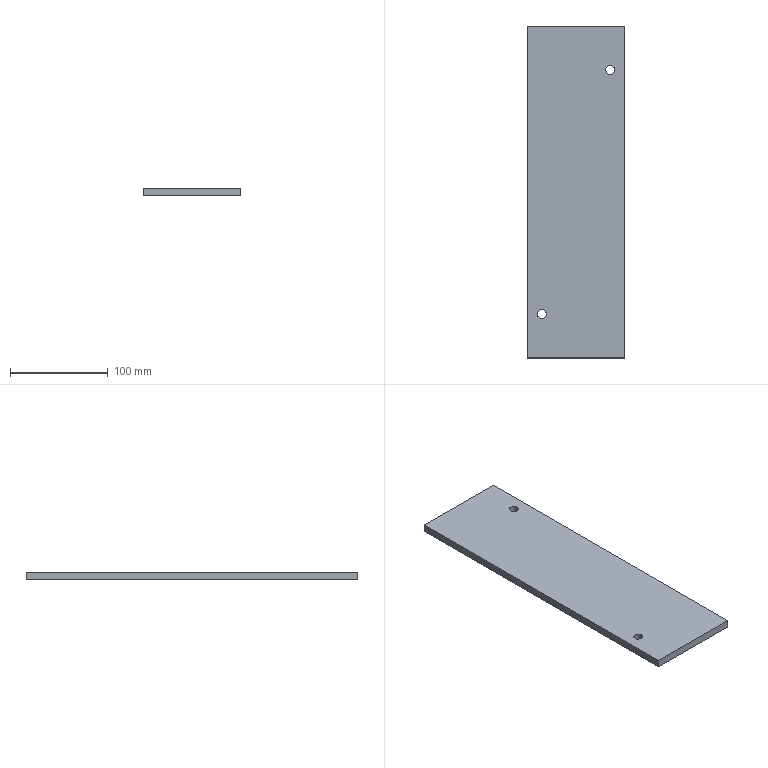Part | SolidWorks | features Extrusion 1, ICE 1 | 1 solid | 10 faces | box 100 x 340 x 8 mm | volume 270982 mm3 | plane 6 | cylinder 4 | commonest cylinder face diameters 9 x4
STEP:
#1=CARTESIAN_POINT('',(-39.5,-125.,-4.));
#2=VERTEX_POINT('',#1);
#3=CARTESIAN_POINT('',(-30.5,-125.,-4.));
#4=VERTEX_POINT('',#3);
#5=CARTESIAN_POINT('',(-35.,-125.,-4.));
#6=DIRECTION('',(0.,0.,1.));
#7=DIRECTION('',(1.,0.,0.));
#8=AXIS2_PLACEMENT_3D('',#5,#6,#7);
#9=CIRCLE('',#8,4.5);
#10=EDGE_CURVE('',#2,#4,#9,.T.);
#11=ORIENTED_EDGE('',*,*,#10,.F.);
#12=CARTESIAN_POINT('',(-39.5,-125.,4.));
#13=VERTEX_POINT('',#12);
#14=CARTESIAN_POINT('',(-39.5,-125.,-14.));
#15=DIRECTION('',(0.,0.,1.));
#16=VECTOR('',#15,1000.);
#17=LINE('',#14,#16);
#18=EDGE_CURVE('',#2,#13,#17,.T.);
#19=ORIENTED_EDGE('',*,*,#18,.T.);
#20=CARTESIAN_POINT('',(-30.5,-125.,4.));
#21=VERTEX_POINT('',#20);
#22=CARTESIAN_POINT('',(-35.,-125.,4.));
#23=DIRECTION('',(0.,0.,1.));
#24=DIRECTION('',(1.,0.,0.));
#25=AXIS2_PLACEMENT_3D('',#22,#23,#24);
#26=CIRCLE('',#25,4.5);
#27=EDGE_CURVE('',#13,#21,#26,.T.);
#28=ORIENTED_EDGE('',*,*,#27,.T.);
#29=CARTESIAN_POINT('',(-30.5,-125.,-14.));
#30=DIRECTION('',(0.,0.,1.));
#31=VECTOR('',#30,1000.);
#32=LINE('',#29,#31);
#33=EDGE_CURVE('',#4,#21,#32,.T.);
#34=ORIENTED_EDGE('',*,*,#33,.F.);
#35=EDGE_LOOP('',(#11,#19,#28,#34));
#36=FACE_OUTER_BOUND('',#35,.T.);
#37=CARTESIAN_POINT('',(-35.,-125.,-14.));
#38=DIRECTION('',(0.,0.,1.));
#39=DIRECTION('',(1.,0.,0.));
#40=AXIS2_PLACEMENT_3D('',#37,#38,#39);
#41=CYLINDRICAL_SURFACE('',#40,4.5);
#42=ADVANCED_FACE('',(#36),#41,.F.);
#43=CARTESIAN_POINT('',(30.5,125.,-4.));
#44=VERTEX_POINT('',#43);
#45=CARTESIAN_POINT('',(39.5,125.,-4.));
#46=VERTEX_POINT('',#45);
#47=CARTESIAN_POINT('',(35.,125.,-4.));
#48=DIRECTION('',(0.,0.,1.));
#49=DIRECTION('',(1.,0.,0.));
#50=AXIS2_PLACEMENT_3D('',#47,#48,#49);
#51=CIRCLE('',#50,4.5);
#52=EDGE_CURVE('',#44,#46,#51,.T.);
#53=ORIENTED_EDGE('',*,*,#52,.F.);
#54=CARTESIAN_POINT('',(30.5,125.,4.));
#55=VERTEX_POINT('',#54);
#56=CARTESIAN_POINT('',(30.5,125.,-14.));
#57=DIRECTION('',(0.,0.,1.));
#58=VECTOR('',#57,1000.);
#59=LINE('',#56,#58);
#60=EDGE_CURVE('',#44,#55,#59,.T.);
#61=ORIENTED_EDGE('',*,*,#60,.T.);
#62=CARTESIAN_POINT('',(39.5,125.,4.));
#63=VERTEX_POINT('',#62);
#64=CARTESIAN_POINT('',(35.,125.,4.));
#65=DIRECTION('',(0.,0.,1.));
#66=DIRECTION('',(1.,0.,0.));
#67=AXIS2_PLACEMENT_3D('',#64,#65,#66);
#68=CIRCLE('',#67,4.5);
#69=EDGE_CURVE('',#55,#63,#68,.T.);
#70=ORIENTED_EDGE('',*,*,#69,.T.);
#71=CARTESIAN_POINT('',(39.5,125.,-14.));
#72=DIRECTION('',(0.,0.,1.));
#73=VECTOR('',#72,1000.);
#74=LINE('',#71,#73);
#75=EDGE_CURVE('',#46,#63,#74,.T.);
#76=ORIENTED_EDGE('',*,*,#75,.F.);
#77=EDGE_LOOP('',(#53,#61,#70,#76));
#78=FACE_OUTER_BOUND('',#77,.T.);
#79=CARTESIAN_POINT('',(35.,125.,-14.));
#80=DIRECTION('',(0.,0.,1.));
#81=DIRECTION('',(1.,0.,0.));
#82=AXIS2_PLACEMENT_3D('',#79,#80,#81);
#83=CYLINDRICAL_SURFACE('',#82,4.5);
#84=ADVANCED_FACE('',(#78),#83,.F.);
#85=CARTESIAN_POINT('',(-50.,170.,4.));
#86=VERTEX_POINT('',#85);
#87=CARTESIAN_POINT('',(-50.,-170.,4.));
#88=VERTEX_POINT('',#87);
#89=CARTESIAN_POINT('',(-50.,170.,4.));
#90=DIRECTION('',(0.,-1.,0.));
#91=VECTOR('',#90,1000.);
#92=LINE('',#89,#91);
#93=EDGE_CURVE('',#86,#88,#92,.T.);
#94=ORIENTED_EDGE('',*,*,#93,.F.);
#95=CARTESIAN_POINT('',(-50.,170.,-4.));
#96=VERTEX_POINT('',#95);
#97=CARTESIAN_POINT('',(-50.,170.,-4.));
#98=DIRECTION('',(0.,0.,1.));
#99=VECTOR('',#98,1000.);
#100=LINE('',#97,#99);
#101=EDGE_CURVE('',#96,#86,#100,.T.);
#102=ORIENTED_EDGE('',*,*,#101,.F.);
#103=CARTESIAN_POINT('',(-50.,-170.,-4.));
#104=VERTEX_POINT('',#103);
#105=CARTESIAN_POINT('',(-50.,170.,-4.));
#106=DIRECTION('',(0.,-1.,0.));
#107=VECTOR('',#106,1000.);
#108=LINE('',#105,#107);
#109=EDGE_CURVE('',#96,#104,#108,.T.);
#110=ORIENTED_EDGE('',*,*,#109,.T.);
#111=CARTESIAN_POINT('',(-50.,-170.,-4.));
#112=DIRECTION('',(0.,0.,1.));
#113=VECTOR('',#112,1000.);
#114=LINE('',#111,#113);
#115=EDGE_CURVE('',#104,#88,#114,.T.);
#116=ORIENTED_EDGE('',*,*,#115,.T.);
#117=EDGE_LOOP('',(#94,#102,#110,#116));
#118=FACE_OUTER_BOUND('',#117,.T.);
#119=CARTESIAN_POINT('',(-50.,170.,-4.));
#120=DIRECTION('',(-1.,0.,0.));
#121=DIRECTION('',(0.,0.,1.));
#122=AXIS2_PLACEMENT_3D('',#119,#120,#121);
#123=PLANE('',#122);
#124=ADVANCED_FACE('',(#118),#123,.T.);
#125=CARTESIAN_POINT('',(50.,170.,4.));
#126=VERTEX_POINT('',#125);
#127=CARTESIAN_POINT('',(50.,170.,4.));
#128=DIRECTION('',(-1.,0.,0.));
#129=VECTOR('',#128,1000.);
#130=LINE('',#127,#129);
#131=EDGE_CURVE('',#126,#86,#130,.T.);
#132=ORIENTED_EDGE('',*,*,#131,.F.);
#133=CARTESIAN_POINT('',(50.,170.,-4.));
#134=VERTEX_POINT('',#133);
#135=CARTESIAN_POINT('',(50.,170.,-4.));
#136=DIRECTION('',(0.,0.,1.));
#137=VECTOR('',#136,1000.);
#138=LINE('',#135,#137);
#139=EDGE_CURVE('',#134,#126,#138,.T.);
#140=ORIENTED_EDGE('',*,*,#139,.F.);
#141=CARTESIAN_POINT('',(50.,170.,-4.));
#142=DIRECTION('',(-1.,0.,0.));
#143=VECTOR('',#142,1000.);
#144=LINE('',#141,#143);
#145=EDGE_CURVE('',#134,#96,#144,.T.);
#146=ORIENTED_EDGE('',*,*,#145,.T.);
#147=ORIENTED_EDGE('',*,*,#101,.T.);
#148=EDGE_LOOP('',(#132,#140,#146,#147));
#149=FACE_OUTER_BOUND('',#148,.T.);
#150=CARTESIAN_POINT('',(50.,170.,-4.));
#151=DIRECTION('',(0.,1.,0.));
#152=DIRECTION('',(0.,0.,1.));
#153=AXIS2_PLACEMENT_3D('',#150,#151,#152);
#154=PLANE('',#153);
#155=ADVANCED_FACE('',(#149),#154,.T.);
#156=CARTESIAN_POINT('',(50.,-170.,4.));
#157=VERTEX_POINT('',#156);
#158=CARTESIAN_POINT('',(50.,-170.,4.));
#159=DIRECTION('',(0.,1.,0.));
#160=VECTOR('',#159,1000.);
#161=LINE('',#158,#160);
#162=EDGE_CURVE('',#157,#126,#161,.T.);
#163=ORIENTED_EDGE('',*,*,#162,.F.);
#164=CARTESIAN_POINT('',(50.,-170.,-4.));
#165=VERTEX_POINT('',#164);
#166=CARTESIAN_POINT('',(50.,-170.,-4.));
#167=DIRECTION('',(0.,0.,1.));
#168=VECTOR('',#167,1000.);
#169=LINE('',#166,#168);
#170=EDGE_CURVE('',#165,#157,#169,.T.);
#171=ORIENTED_EDGE('',*,*,#170,.F.);
#172=CARTESIAN_POINT('',(50.,-170.,-4.));
#173=DIRECTION('',(0.,1.,0.));
#174=VECTOR('',#173,1000.);
#175=LINE('',#172,#174);
#176=EDGE_CURVE('',#165,#134,#175,.T.);
#177=ORIENTED_EDGE('',*,*,#176,.T.);
#178=ORIENTED_EDGE('',*,*,#139,.T.);
#179=EDGE_LOOP('',(#163,#171,#177,#178));
#180=FACE_OUTER_BOUND('',#179,.T.);
#181=CARTESIAN_POINT('',(50.,-170.,-4.));
#182=DIRECTION('',(1.,0.,0.));
#183=DIRECTION('',(0.,0.,-1.));
#184=AXIS2_PLACEMENT_3D('',#181,#182,#183);
#185=PLANE('',#184);
#186=ADVANCED_FACE('',(#180),#185,.T.);
#187=CARTESIAN_POINT('',(-50.,-170.,4.));
#188=DIRECTION('',(1.,0.,0.));
#189=VECTOR('',#188,1000.);
#190=LINE('',#187,#189);
#191=EDGE_CURVE('',#88,#157,#190,.T.);
#192=ORIENTED_EDGE('',*,*,#191,.F.);
#193=ORIENTED_EDGE('',*,*,#115,.F.);
#194=CARTESIAN_POINT('',(-50.,-170.,-4.));
#195=DIRECTION('',(1.,0.,0.));
#196=VECTOR('',#195,1000.);
#197=LINE('',#194,#196);
#198=EDGE_CURVE('',#104,#165,#197,.T.);
#199=ORIENTED_EDGE('',*,*,#198,.T.);
#200=ORIENTED_EDGE('',*,*,#170,.T.);
#201=EDGE_LOOP('',(#192,#193,#199,#200));
#202=FACE_OUTER_BOUND('',#201,.T.);
#203=CARTESIAN_POINT('',(-50.,-170.,-4.));
#204=DIRECTION('',(0.,-1.,0.));
#205=DIRECTION('',(0.,0.,-1.));
#206=AXIS2_PLACEMENT_3D('',#203,#204,#205);
#207=PLANE('',#206);
#208=ADVANCED_FACE('',(#202),#207,.T.);
#209=CARTESIAN_POINT('',(-35.,-125.,-4.));
#210=DIRECTION('',(0.,0.,1.));
#211=DIRECTION('',(1.,0.,0.));
#212=AXIS2_PLACEMENT_3D('',#209,#210,#211);
#213=CIRCLE('',#212,4.5);
#214=EDGE_CURVE('',#4,#2,#213,.T.);
#215=ORIENTED_EDGE('',*,*,#214,.T.);
#216=ORIENTED_EDGE('',*,*,#10,.T.);
#217=EDGE_LOOP('',(#215,#216));
#218=FACE_BOUND('',#217,.T.);
#219=CARTESIAN_POINT('',(35.,125.,-4.));
#220=DIRECTION('',(0.,0.,1.));
#221=DIRECTION('',(1.,0.,0.));
#222=AXIS2_PLACEMENT_3D('',#219,#220,#221);
#223=CIRCLE('',#222,4.5);
#224=EDGE_CURVE('',#46,#44,#223,.T.);
#225=ORIENTED_EDGE('',*,*,#224,.T.);
#226=ORIENTED_EDGE('',*,*,#52,.T.);
#227=EDGE_LOOP('',(#225,#226));
#228=FACE_BOUND('',#227,.T.);
#229=ORIENTED_EDGE('',*,*,#109,.F.);
#230=ORIENTED_EDGE('',*,*,#145,.F.);
#231=ORIENTED_EDGE('',*,*,#176,.F.);
#232=ORIENTED_EDGE('',*,*,#198,.F.);
#233=EDGE_LOOP('',(#229,#230,#231,#232));
#234=FACE_OUTER_BOUND('',#233,.T.);
#235=CARTESIAN_POINT('',(0.,0.,-4.));
#236=DIRECTION('',(0.,0.,1.));
#237=DIRECTION('',(1.,0.,0.));
#238=AXIS2_PLACEMENT_3D('',#235,#236,#237);
#239=PLANE('',#238);
#240=ADVANCED_FACE('',(#218,#228,#234),#239,.F.);
#241=CARTESIAN_POINT('',(-35.,-125.,4.));
#242=DIRECTION('',(0.,0.,1.));
#243=DIRECTION('',(1.,0.,0.));
#244=AXIS2_PLACEMENT_3D('',#241,#242,#243);
#245=CIRCLE('',#244,4.5);
#246=EDGE_CURVE('',#21,#13,#245,.T.);
#247=ORIENTED_EDGE('',*,*,#246,.F.);
#248=ORIENTED_EDGE('',*,*,#27,.F.);
#249=EDGE_LOOP('',(#247,#248));
#250=FACE_BOUND('',#249,.T.);
#251=CARTESIAN_POINT('',(35.,125.,4.));
#252=DIRECTION('',(0.,0.,1.));
#253=DIRECTION('',(1.,0.,0.));
#254=AXIS2_PLACEMENT_3D('',#251,#252,#253);
#255=CIRCLE('',#254,4.5);
#256=EDGE_CURVE('',#63,#55,#255,.T.);
#257=ORIENTED_EDGE('',*,*,#256,.F.);
#258=ORIENTED_EDGE('',*,*,#69,.F.);
#259=EDGE_LOOP('',(#257,#258));
#260=FACE_BOUND('',#259,.T.);
#261=ORIENTED_EDGE('',*,*,#93,.T.);
#262=ORIENTED_EDGE('',*,*,#191,.T.);
#263=ORIENTED_EDGE('',*,*,#162,.T.);
#264=ORIENTED_EDGE('',*,*,#131,.T.);
#265=EDGE_LOOP('',(#261,#262,#263,#264));
#266=FACE_OUTER_BOUND('',#265,.T.);
#267=CARTESIAN_POINT('',(0.,0.,4.));
#268=DIRECTION('',(0.,0.,1.));
#269=DIRECTION('',(1.,0.,0.));
#270=AXIS2_PLACEMENT_3D('',#267,#268,#269);
#271=PLANE('',#270);
#272=ADVANCED_FACE('',(#250,#260,#266),#271,.T.);
#273=ORIENTED_EDGE('',*,*,#60,.F.);
#274=ORIENTED_EDGE('',*,*,#224,.F.);
#275=ORIENTED_EDGE('',*,*,#75,.T.);
#276=ORIENTED_EDGE('',*,*,#256,.T.);
#277=EDGE_LOOP('',(#273,#274,#275,#276));
#278=FACE_OUTER_BOUND('',#277,.T.);
#279=CARTESIAN_POINT('',(35.,125.,-14.));
#280=DIRECTION('',(0.,0.,1.));
#281=DIRECTION('',(1.,0.,0.));
#282=AXIS2_PLACEMENT_3D('',#279,#280,#281);
#283=CYLINDRICAL_SURFACE('',#282,4.5);
#284=ADVANCED_FACE('',(#278),#283,.F.);
#285=ORIENTED_EDGE('',*,*,#18,.F.);
#286=ORIENTED_EDGE('',*,*,#214,.F.);
#287=ORIENTED_EDGE('',*,*,#33,.T.);
#288=ORIENTED_EDGE('',*,*,#246,.T.);
#289=EDGE_LOOP('',(#285,#286,#287,#288));
#290=FACE_OUTER_BOUND('',#289,.T.);
#291=CARTESIAN_POINT('',(-35.,-125.,-14.));
#292=DIRECTION('',(0.,0.,1.));
#293=DIRECTION('',(1.,0.,0.));
#294=AXIS2_PLACEMENT_3D('',#291,#292,#293);
#295=CYLINDRICAL_SURFACE('',#294,4.5);
#296=ADVANCED_FACE('',(#290),#295,.F.);
#297=CLOSED_SHELL('',(#42,#84,#124,#155,#186,#208,#240,#272,#284,#296));
#298=MANIFOLD_SOLID_BREP('',#297);
#299=CARTESIAN_POINT('',(0.,0.,0.));
#300=DIRECTION('',(0.,0.,1.));
#301=DIRECTION('',(1.,0.,0.));
#302=AXIS2_PLACEMENT_3D('',#299,#300,#301);
#303=(LENGTH_UNIT()NAMED_UNIT(*)SI_UNIT(.MILLI.,.METRE.));
#304=UNCERTAINTY_MEASURE_WITH_UNIT(LENGTH_MEASURE(0.00001),#303,'','');
#305=(NAMED_UNIT(*)PLANE_ANGLE_UNIT()SI_UNIT($,.RADIAN.));
#306=(NAMED_UNIT(*)SI_UNIT($,.STERADIAN.)SOLID_ANGLE_UNIT());
#307=(GEOMETRIC_REPRESENTATION_CONTEXT(3)GLOBAL_UNCERTAINTY_ASSIGNED_CONTEXT((#304))GLOBAL_UNIT_ASSIGNED_CONTEXT((#303,#305,#306))REPRESENTATION_CONTEXT('',''));
#308=ADVANCED_BREP_SHAPE_REPRESENTATION('',(#298,#302),#307);